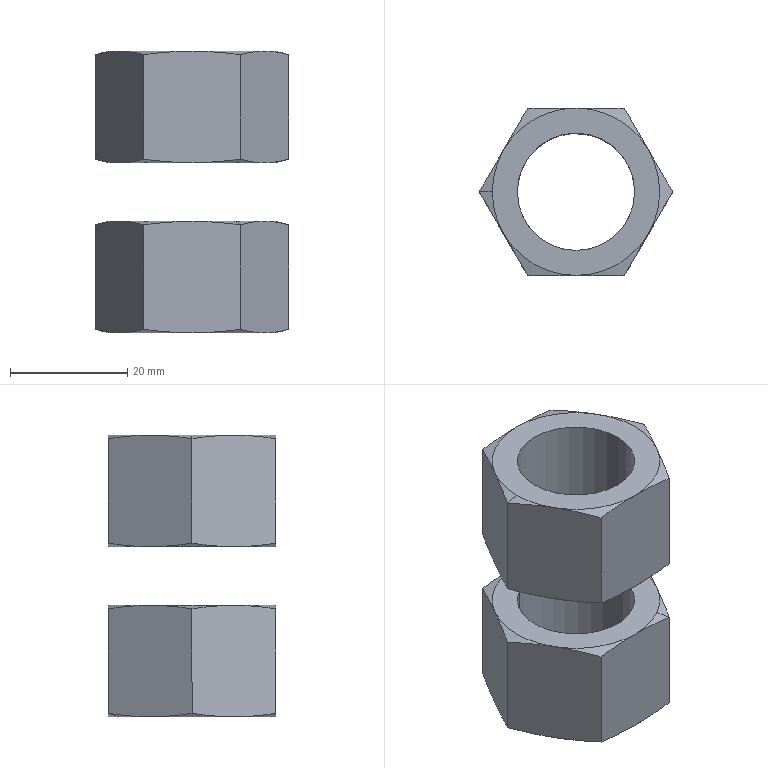Part | NX | features BREP 1 | 2 solids | 48 faces | box 32.95 x 28.536 x 48 mm | volume 14812 mm3 | cone 28 | plane 16 | cylinder 4 | commonest cylinder face diameters 20 x4